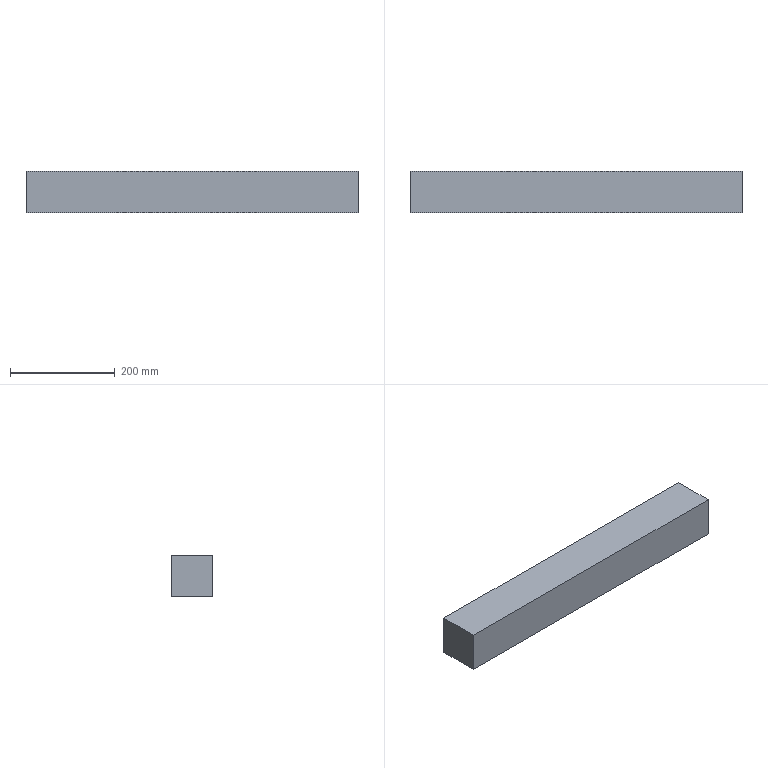Part | STEP file | Crossbeam | 1 solid | 12 faces | box 635 x 80 x 80 mm | volume 1850000 mm3 | plane 12
STEP:
#1=CARTESIAN_POINT('',(-635.,0.,0.));
#2=VERTEX_POINT('',#1);
#3=CARTESIAN_POINT('',(0.,0.,0.));
#4=VERTEX_POINT('',#3);
#5=CARTESIAN_POINT('',(0.,0.,0.));
#6=DIRECTION('',(1.,0.,0.));
#7=VECTOR('',#6,1000.);
#8=LINE('',#5,#7);
#9=EDGE_CURVE('',#2,#4,#8,.T.);
#10=ORIENTED_EDGE('',*,*,#9,.T.);
#11=CARTESIAN_POINT('',(0.,0.,80.));
#12=VERTEX_POINT('',#11);
#13=CARTESIAN_POINT('',(0.,0.,80.));
#14=DIRECTION('',(0.,0.,-1.));
#15=VECTOR('',#14,1000.);
#16=LINE('',#13,#15);
#17=EDGE_CURVE('',#12,#4,#16,.T.);
#18=ORIENTED_EDGE('',*,*,#17,.F.);
#19=CARTESIAN_POINT('',(-635.,0.,80.));
#20=VERTEX_POINT('',#19);
#21=CARTESIAN_POINT('',(0.,0.,80.));
#22=DIRECTION('',(1.,0.,0.));
#23=VECTOR('',#22,1000.);
#24=LINE('',#21,#23);
#25=EDGE_CURVE('',#20,#12,#24,.T.);
#26=ORIENTED_EDGE('',*,*,#25,.F.);
#27=CARTESIAN_POINT('',(-635.,0.,80.));
#28=DIRECTION('',(0.,0.,-1.));
#29=VECTOR('',#28,1000.);
#30=LINE('',#27,#29);
#31=EDGE_CURVE('',#20,#2,#30,.T.);
#32=ORIENTED_EDGE('',*,*,#31,.T.);
#33=EDGE_LOOP('',(#10,#18,#26,#32));
#34=FACE_OUTER_BOUND('',#33,.T.);
#35=CARTESIAN_POINT('',(0.,0.,80.));
#36=DIRECTION('',(0.,1.,0.));
#37=DIRECTION('',(-1.,0.,0.));
#38=AXIS2_PLACEMENT_3D('',#35,#36,#37);
#39=PLANE('',#38);
#40=ADVANCED_FACE('',(#34),#39,.F.);
#41=CARTESIAN_POINT('',(0.,80.,0.));
#42=VERTEX_POINT('',#41);
#43=CARTESIAN_POINT('',(0.,0.,0.));
#44=DIRECTION('',(0.,1.,0.));
#45=VECTOR('',#44,1000.);
#46=LINE('',#43,#45);
#47=EDGE_CURVE('',#4,#42,#46,.T.);
#48=ORIENTED_EDGE('',*,*,#47,.T.);
#49=CARTESIAN_POINT('',(0.,80.,80.));
#50=VERTEX_POINT('',#49);
#51=CARTESIAN_POINT('',(0.,80.,80.));
#52=DIRECTION('',(0.,0.,-1.));
#53=VECTOR('',#52,1000.);
#54=LINE('',#51,#53);
#55=EDGE_CURVE('',#50,#42,#54,.T.);
#56=ORIENTED_EDGE('',*,*,#55,.F.);
#57=CARTESIAN_POINT('',(0.,0.,80.));
#58=DIRECTION('',(0.,1.,0.));
#59=VECTOR('',#58,1000.);
#60=LINE('',#57,#59);
#61=EDGE_CURVE('',#12,#50,#60,.T.);
#62=ORIENTED_EDGE('',*,*,#61,.F.);
#63=ORIENTED_EDGE('',*,*,#17,.T.);
#64=EDGE_LOOP('',(#48,#56,#62,#63));
#65=FACE_OUTER_BOUND('',#64,.T.);
#66=CARTESIAN_POINT('',(0.,0.,80.));
#67=DIRECTION('',(-1.,0.,0.));
#68=DIRECTION('',(0.,0.,1.));
#69=AXIS2_PLACEMENT_3D('',#66,#67,#68);
#70=PLANE('',#69);
#71=ADVANCED_FACE('',(#65),#70,.F.);
#72=CARTESIAN_POINT('',(-635.,80.,0.));
#73=VERTEX_POINT('',#72);
#74=CARTESIAN_POINT('',(0.,80.,0.));
#75=DIRECTION('',(-1.,0.,0.));
#76=VECTOR('',#75,1000.);
#77=LINE('',#74,#76);
#78=EDGE_CURVE('',#42,#73,#77,.T.);
#79=ORIENTED_EDGE('',*,*,#78,.T.);
#80=CARTESIAN_POINT('',(-635.,80.,80.));
#81=VERTEX_POINT('',#80);
#82=CARTESIAN_POINT('',(-635.,80.,80.));
#83=DIRECTION('',(0.,0.,-1.));
#84=VECTOR('',#83,1000.);
#85=LINE('',#82,#84);
#86=EDGE_CURVE('',#81,#73,#85,.T.);
#87=ORIENTED_EDGE('',*,*,#86,.F.);
#88=CARTESIAN_POINT('',(0.,80.,80.));
#89=DIRECTION('',(-1.,0.,0.));
#90=VECTOR('',#89,1000.);
#91=LINE('',#88,#90);
#92=EDGE_CURVE('',#50,#81,#91,.T.);
#93=ORIENTED_EDGE('',*,*,#92,.F.);
#94=ORIENTED_EDGE('',*,*,#55,.T.);
#95=EDGE_LOOP('',(#79,#87,#93,#94));
#96=FACE_OUTER_BOUND('',#95,.T.);
#97=CARTESIAN_POINT('',(0.,80.,80.));
#98=DIRECTION('',(0.,-1.,0.));
#99=DIRECTION('',(1.,0.,0.));
#100=AXIS2_PLACEMENT_3D('',#97,#98,#99);
#101=PLANE('',#100);
#102=ADVANCED_FACE('',(#96),#101,.F.);
#103=CARTESIAN_POINT('',(-635.,80.,0.));
#104=DIRECTION('',(0.,-1.,0.));
#105=VECTOR('',#104,1000.);
#106=LINE('',#103,#105);
#107=EDGE_CURVE('',#73,#2,#106,.T.);
#108=ORIENTED_EDGE('',*,*,#107,.T.);
#109=ORIENTED_EDGE('',*,*,#31,.F.);
#110=CARTESIAN_POINT('',(-635.,80.,80.));
#111=DIRECTION('',(0.,-1.,0.));
#112=VECTOR('',#111,1000.);
#113=LINE('',#110,#112);
#114=EDGE_CURVE('',#81,#20,#113,.T.);
#115=ORIENTED_EDGE('',*,*,#114,.F.);
#116=ORIENTED_EDGE('',*,*,#86,.T.);
#117=EDGE_LOOP('',(#108,#109,#115,#116));
#118=FACE_OUTER_BOUND('',#117,.T.);
#119=CARTESIAN_POINT('',(-635.,80.,80.));
#120=DIRECTION('',(1.,0.,0.));
#121=DIRECTION('',(0.,0.,-1.));
#122=AXIS2_PLACEMENT_3D('',#119,#120,#121);
#123=PLANE('',#122);
#124=ADVANCED_FACE('',(#118),#123,.F.);
#125=ORIENTED_EDGE('',*,*,#25,.T.);
#126=ORIENTED_EDGE('',*,*,#61,.T.);
#127=ORIENTED_EDGE('',*,*,#92,.T.);
#128=ORIENTED_EDGE('',*,*,#114,.T.);
#129=EDGE_LOOP('',(#125,#126,#127,#128));
#130=FACE_OUTER_BOUND('',#129,.T.);
#131=CARTESIAN_POINT('',(0.,0.,80.));
#132=DIRECTION('',(0.,0.,1.));
#133=DIRECTION('',(1.,0.,0.));
#134=AXIS2_PLACEMENT_3D('',#131,#132,#133);
#135=PLANE('',#134);
#136=ADVANCED_FACE('',(#130),#135,.T.);
#137=ORIENTED_EDGE('',*,*,#9,.F.);
#138=ORIENTED_EDGE('',*,*,#107,.F.);
#139=ORIENTED_EDGE('',*,*,#78,.F.);
#140=ORIENTED_EDGE('',*,*,#47,.F.);
#141=EDGE_LOOP('',(#137,#138,#139,#140));
#142=FACE_OUTER_BOUND('',#141,.T.);
#143=CARTESIAN_POINT('',(0.,0.,0.));
#144=DIRECTION('',(0.,0.,1.));
#145=DIRECTION('',(1.,0.,0.));
#146=AXIS2_PLACEMENT_3D('',#143,#144,#145);
#147=PLANE('',#146);
#148=ADVANCED_FACE('',(#142),#147,.F.);
#149=CLOSED_SHELL('',(#40,#71,#102,#124,#136,#148));
#150=CARTESIAN_POINT('',(-625.,10.,10.));
#151=VERTEX_POINT('',#150);
#152=CARTESIAN_POINT('',(-10.,10.,10.));
#153=VERTEX_POINT('',#152);
#154=CARTESIAN_POINT('',(0.,10.,10.));
#155=DIRECTION('',(1.,0.,0.));
#156=VECTOR('',#155,1000.);
#157=LINE('',#154,#156);
#158=EDGE_CURVE('',#151,#153,#157,.T.);
#159=ORIENTED_EDGE('',*,*,#158,.F.);
#160=CARTESIAN_POINT('',(-625.,10.,70.));
#161=VERTEX_POINT('',#160);
#162=CARTESIAN_POINT('',(-625.,10.,80.));
#163=DIRECTION('',(0.,0.,-1.));
#164=VECTOR('',#163,1000.);
#165=LINE('',#162,#164);
#166=EDGE_CURVE('',#161,#151,#165,.T.);
#167=ORIENTED_EDGE('',*,*,#166,.F.);
#168=CARTESIAN_POINT('',(-10.,10.,70.));
#169=VERTEX_POINT('',#168);
#170=CARTESIAN_POINT('',(0.,10.,70.));
#171=DIRECTION('',(1.,0.,0.));
#172=VECTOR('',#171,1000.);
#173=LINE('',#170,#172);
#174=EDGE_CURVE('',#161,#169,#173,.T.);
#175=ORIENTED_EDGE('',*,*,#174,.T.);
#176=CARTESIAN_POINT('',(-10.,10.,80.));
#177=DIRECTION('',(0.,0.,-1.));
#178=VECTOR('',#177,1000.);
#179=LINE('',#176,#178);
#180=EDGE_CURVE('',#169,#153,#179,.T.);
#181=ORIENTED_EDGE('',*,*,#180,.T.);
#182=EDGE_LOOP('',(#159,#167,#175,#181));
#183=FACE_OUTER_BOUND('',#182,.T.);
#184=CARTESIAN_POINT('',(0.,10.,80.));
#185=DIRECTION('',(0.,1.,0.));
#186=DIRECTION('',(-1.,0.,0.));
#187=AXIS2_PLACEMENT_3D('',#184,#185,#186);
#188=PLANE('',#187);
#189=ADVANCED_FACE('',(#183),#188,.T.);
#190=CARTESIAN_POINT('',(-10.,70.,10.));
#191=VERTEX_POINT('',#190);
#192=CARTESIAN_POINT('',(-10.,0.,10.));
#193=DIRECTION('',(0.,1.,0.));
#194=VECTOR('',#193,1000.);
#195=LINE('',#192,#194);
#196=EDGE_CURVE('',#153,#191,#195,.T.);
#197=ORIENTED_EDGE('',*,*,#196,.F.);
#198=ORIENTED_EDGE('',*,*,#180,.F.);
#199=CARTESIAN_POINT('',(-10.,70.,70.));
#200=VERTEX_POINT('',#199);
#201=CARTESIAN_POINT('',(-10.,0.,70.));
#202=DIRECTION('',(0.,1.,0.));
#203=VECTOR('',#202,1000.);
#204=LINE('',#201,#203);
#205=EDGE_CURVE('',#169,#200,#204,.T.);
#206=ORIENTED_EDGE('',*,*,#205,.T.);
#207=CARTESIAN_POINT('',(-10.,70.,80.));
#208=DIRECTION('',(0.,0.,-1.));
#209=VECTOR('',#208,1000.);
#210=LINE('',#207,#209);
#211=EDGE_CURVE('',#200,#191,#210,.T.);
#212=ORIENTED_EDGE('',*,*,#211,.T.);
#213=EDGE_LOOP('',(#197,#198,#206,#212));
#214=FACE_OUTER_BOUND('',#213,.T.);
#215=CARTESIAN_POINT('',(-10.,0.,80.));
#216=DIRECTION('',(-1.,0.,0.));
#217=DIRECTION('',(0.,0.,1.));
#218=AXIS2_PLACEMENT_3D('',#215,#216,#217);
#219=PLANE('',#218);
#220=ADVANCED_FACE('',(#214),#219,.T.);
#221=CARTESIAN_POINT('',(-625.,70.,10.));
#222=VERTEX_POINT('',#221);
#223=CARTESIAN_POINT('',(0.,70.,10.));
#224=DIRECTION('',(-1.,0.,0.));
#225=VECTOR('',#224,1000.);
#226=LINE('',#223,#225);
#227=EDGE_CURVE('',#191,#222,#226,.T.);
#228=ORIENTED_EDGE('',*,*,#227,.F.);
#229=ORIENTED_EDGE('',*,*,#211,.F.);
#230=CARTESIAN_POINT('',(-625.,70.,70.));
#231=VERTEX_POINT('',#230);
#232=CARTESIAN_POINT('',(0.,70.,70.));
#233=DIRECTION('',(-1.,0.,0.));
#234=VECTOR('',#233,1000.);
#235=LINE('',#232,#234);
#236=EDGE_CURVE('',#200,#231,#235,.T.);
#237=ORIENTED_EDGE('',*,*,#236,.T.);
#238=CARTESIAN_POINT('',(-625.,70.,80.));
#239=DIRECTION('',(0.,0.,-1.));
#240=VECTOR('',#239,1000.);
#241=LINE('',#238,#240);
#242=EDGE_CURVE('',#231,#222,#241,.T.);
#243=ORIENTED_EDGE('',*,*,#242,.T.);
#244=EDGE_LOOP('',(#228,#229,#237,#243));
#245=FACE_OUTER_BOUND('',#244,.T.);
#246=CARTESIAN_POINT('',(0.,70.,80.));
#247=DIRECTION('',(0.,-1.,0.));
#248=DIRECTION('',(1.,0.,0.));
#249=AXIS2_PLACEMENT_3D('',#246,#247,#248);
#250=PLANE('',#249);
#251=ADVANCED_FACE('',(#245),#250,.T.);
#252=CARTESIAN_POINT('',(-625.,80.,10.));
#253=DIRECTION('',(0.,-1.,0.));
#254=VECTOR('',#253,1000.);
#255=LINE('',#252,#254);
#256=EDGE_CURVE('',#222,#151,#255,.T.);
#257=ORIENTED_EDGE('',*,*,#256,.F.);
#258=ORIENTED_EDGE('',*,*,#242,.F.);
#259=CARTESIAN_POINT('',(-625.,80.,70.));
#260=DIRECTION('',(0.,-1.,0.));
#261=VECTOR('',#260,1000.);
#262=LINE('',#259,#261);
#263=EDGE_CURVE('',#231,#161,#262,.T.);
#264=ORIENTED_EDGE('',*,*,#263,.T.);
#265=ORIENTED_EDGE('',*,*,#166,.T.);
#266=EDGE_LOOP('',(#257,#258,#264,#265));
#267=FACE_OUTER_BOUND('',#266,.T.);
#268=CARTESIAN_POINT('',(-625.,80.,80.));
#269=DIRECTION('',(1.,0.,0.));
#270=DIRECTION('',(0.,0.,-1.));
#271=AXIS2_PLACEMENT_3D('',#268,#269,#270);
#272=PLANE('',#271);
#273=ADVANCED_FACE('',(#267),#272,.T.);
#274=ORIENTED_EDGE('',*,*,#174,.F.);
#275=ORIENTED_EDGE('',*,*,#263,.F.);
#276=ORIENTED_EDGE('',*,*,#236,.F.);
#277=ORIENTED_EDGE('',*,*,#205,.F.);
#278=EDGE_LOOP('',(#274,#275,#276,#277));
#279=FACE_OUTER_BOUND('',#278,.T.);
#280=CARTESIAN_POINT('',(0.,0.,70.));
#281=DIRECTION('',(0.,0.,1.));
#282=DIRECTION('',(1.,0.,0.));
#283=AXIS2_PLACEMENT_3D('',#280,#281,#282);
#284=PLANE('',#283);
#285=ADVANCED_FACE('',(#279),#284,.F.);
#286=ORIENTED_EDGE('',*,*,#158,.T.);
#287=ORIENTED_EDGE('',*,*,#196,.T.);
#288=ORIENTED_EDGE('',*,*,#227,.T.);
#289=ORIENTED_EDGE('',*,*,#256,.T.);
#290=EDGE_LOOP('',(#286,#287,#288,#289));
#291=FACE_OUTER_BOUND('',#290,.T.);
#292=CARTESIAN_POINT('',(0.,0.,10.));
#293=DIRECTION('',(0.,0.,1.));
#294=DIRECTION('',(1.,0.,0.));
#295=AXIS2_PLACEMENT_3D('',#292,#293,#294);
#296=PLANE('',#295);
#297=ADVANCED_FACE('',(#291),#296,.T.);
#298=CLOSED_SHELL('',(#189,#220,#251,#273,#285,#297));
#299=ORIENTED_CLOSED_SHELL('',*,#298,.F.);
#300=BREP_WITH_VOIDS('',#149,(#299));
#301=CARTESIAN_POINT('',(0.,0.,0.));
#302=DIRECTION('',(0.,0.,1.));
#303=DIRECTION('',(1.,0.,0.));
#304=AXIS2_PLACEMENT_3D('',#301,#302,#303);
#305=(LENGTH_UNIT()NAMED_UNIT(*)SI_UNIT(.MILLI.,.METRE.));
#306=UNCERTAINTY_MEASURE_WITH_UNIT(LENGTH_MEASURE(0.00001),#305,'','');
#307=(NAMED_UNIT(*)PLANE_ANGLE_UNIT()SI_UNIT($,.RADIAN.));
#308=(NAMED_UNIT(*)SI_UNIT($,.STERADIAN.)SOLID_ANGLE_UNIT());
#309=(GEOMETRIC_REPRESENTATION_CONTEXT(3)GLOBAL_UNCERTAINTY_ASSIGNED_CONTEXT((#306))GLOBAL_UNIT_ASSIGNED_CONTEXT((#305,#307,#308))REPRESENTATION_CONTEXT('',''));
#310=ADVANCED_BREP_SHAPE_REPRESENTATION('',(#300,#304),#309);